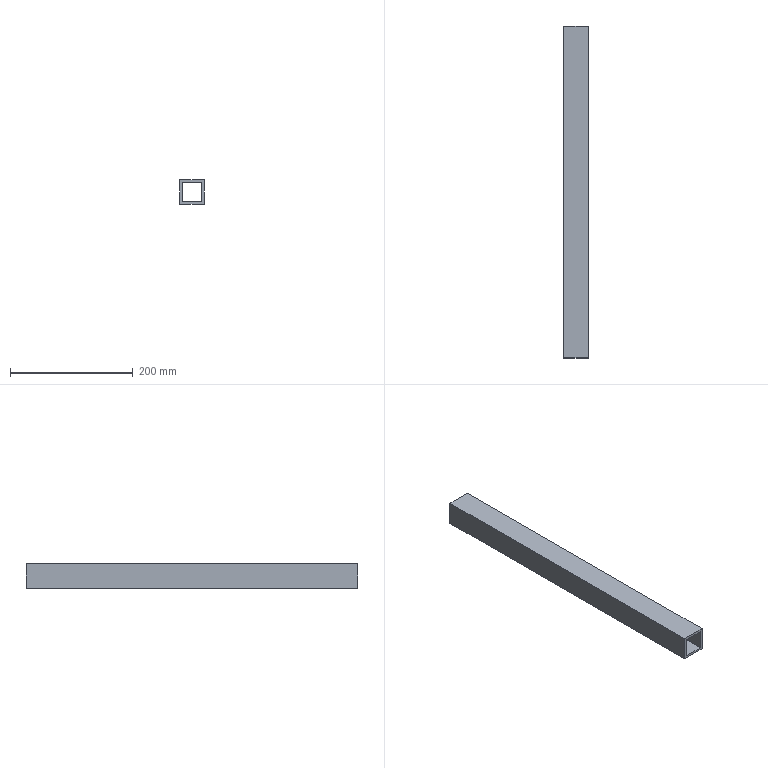Part | NX | features solid 2 | 1 solid | 10 faces | box 40 x 540 x 40 mm | volume 311040 mm3 | plane 10
STEP:
#1=CARTESIAN_POINT('',(-1540.,-370.,-85.));
#2=VERTEX_POINT('',#1);
#3=CARTESIAN_POINT('',(-1540.,170.,-85.));
#4=VERTEX_POINT('',#3);
#5=CARTESIAN_POINT('',(-1540.,1629.393,-85.));
#6=DIRECTION('',(0.,1.,0.));
#7=VECTOR('',#6,1000.);
#8=LINE('',#5,#7);
#9=EDGE_CURVE('',#2,#4,#8,.T.);
#10=ORIENTED_EDGE('',*,*,#9,.T.);
#11=CARTESIAN_POINT('',(-1540.,170.,-45.));
#12=VERTEX_POINT('',#11);
#13=CARTESIAN_POINT('',(-1540.,170.,-70.));
#14=DIRECTION('',(0.,0.,1.));
#15=VECTOR('',#14,1000.);
#16=LINE('',#13,#15);
#17=EDGE_CURVE('',#4,#12,#16,.T.);
#18=ORIENTED_EDGE('',*,*,#17,.T.);
#19=CARTESIAN_POINT('',(-1540.,-370.,-45.));
#20=VERTEX_POINT('',#19);
#21=CARTESIAN_POINT('',(-1540.,1714.393,-45.));
#22=DIRECTION('',(0.,1.,0.));
#23=VECTOR('',#22,1000.);
#24=LINE('',#21,#23);
#25=EDGE_CURVE('',#20,#12,#24,.T.);
#26=ORIENTED_EDGE('',*,*,#25,.F.);
#27=CARTESIAN_POINT('',(-1540.,-370.,-70.));
#28=DIRECTION('',(0.,0.,-1.));
#29=VECTOR('',#28,1000.);
#30=LINE('',#27,#29);
#31=EDGE_CURVE('',#20,#2,#30,.T.);
#32=ORIENTED_EDGE('',*,*,#31,.T.);
#33=EDGE_LOOP('',(#10,#18,#26,#32));
#34=FACE_BOUND('',#33,.T.);
#35=CARTESIAN_POINT('',(-1540.,1629.393,-70.));
#36=DIRECTION('',(-1.,0.,0.));
#37=DIRECTION('',(0.,0.,1.));
#38=AXIS2_PLACEMENT_3D('',#35,#36,#37);
#39=PLANE('',#38);
#40=ADVANCED_FACE('',(#34),#39,.F.);
#41=CARTESIAN_POINT('',(-1580.,-370.,-85.));
#42=VERTEX_POINT('',#41);
#43=CARTESIAN_POINT('',(-1580.,170.,-85.));
#44=VERTEX_POINT('',#43);
#45=CARTESIAN_POINT('',(-1580.,1714.393,-85.));
#46=DIRECTION('',(0.,1.,0.));
#47=VECTOR('',#46,1000.);
#48=LINE('',#45,#47);
#49=EDGE_CURVE('',#42,#44,#48,.T.);
#50=ORIENTED_EDGE('',*,*,#49,.T.);
#51=CARTESIAN_POINT('',(-960.,170.,-85.));
#52=DIRECTION('',(1.,0.,0.));
#53=VECTOR('',#52,1000.);
#54=LINE('',#51,#53);
#55=EDGE_CURVE('',#44,#4,#54,.T.);
#56=ORIENTED_EDGE('',*,*,#55,.T.);
#57=ORIENTED_EDGE('',*,*,#9,.F.);
#58=CARTESIAN_POINT('',(-960.,-370.,-85.));
#59=DIRECTION('',(-1.,0.,0.));
#60=VECTOR('',#59,1000.);
#61=LINE('',#58,#60);
#62=EDGE_CURVE('',#2,#42,#61,.T.);
#63=ORIENTED_EDGE('',*,*,#62,.T.);
#64=EDGE_LOOP('',(#50,#56,#57,#63));
#65=FACE_BOUND('',#64,.T.);
#66=CARTESIAN_POINT('',(-960.,1714.393,-85.));
#67=DIRECTION('',(0.,0.,1.));
#68=DIRECTION('',(1.,0.,0.));
#69=AXIS2_PLACEMENT_3D('',#66,#67,#68);
#70=PLANE('',#69);
#71=ADVANCED_FACE('',(#65),#70,.F.);
#72=ORIENTED_EDGE('',*,*,#25,.T.);
#73=CARTESIAN_POINT('',(-1580.,170.,-45.));
#74=VERTEX_POINT('',#73);
#75=CARTESIAN_POINT('',(-920.,170.,-45.));
#76=DIRECTION('',(-1.,0.,0.));
#77=VECTOR('',#76,1000.);
#78=LINE('',#75,#77);
#79=EDGE_CURVE('',#12,#74,#78,.T.);
#80=ORIENTED_EDGE('',*,*,#79,.T.);
#81=CARTESIAN_POINT('',(-1580.,-370.,-45.));
#82=VERTEX_POINT('',#81);
#83=CARTESIAN_POINT('',(-1580.,1714.393,-45.));
#84=DIRECTION('',(0.,-1.,0.));
#85=VECTOR('',#84,1000.);
#86=LINE('',#83,#85);
#87=EDGE_CURVE('',#74,#82,#86,.T.);
#88=ORIENTED_EDGE('',*,*,#87,.T.);
#89=CARTESIAN_POINT('',(-920.,-370.,-45.));
#90=DIRECTION('',(1.,0.,0.));
#91=VECTOR('',#90,1000.);
#92=LINE('',#89,#91);
#93=EDGE_CURVE('',#82,#20,#92,.T.);
#94=ORIENTED_EDGE('',*,*,#93,.T.);
#95=EDGE_LOOP('',(#72,#80,#88,#94));
#96=FACE_BOUND('',#95,.T.);
#97=CARTESIAN_POINT('',(-920.,1714.393,-45.));
#98=DIRECTION('',(0.,0.,-1.));
#99=DIRECTION('',(-1.,0.,0.));
#100=AXIS2_PLACEMENT_3D('',#97,#98,#99);
#101=PLANE('',#100);
#102=ADVANCED_FACE('',(#96),#101,.F.);
#103=ORIENTED_EDGE('',*,*,#87,.F.);
#104=CARTESIAN_POINT('',(-1580.,170.,-40.));
#105=DIRECTION('',(0.,0.,-1.));
#106=VECTOR('',#105,1000.);
#107=LINE('',#104,#106);
#108=EDGE_CURVE('',#74,#44,#107,.T.);
#109=ORIENTED_EDGE('',*,*,#108,.T.);
#110=ORIENTED_EDGE('',*,*,#49,.F.);
#111=CARTESIAN_POINT('',(-1580.,-370.,-40.));
#112=DIRECTION('',(0.,0.,1.));
#113=VECTOR('',#112,1000.);
#114=LINE('',#111,#113);
#115=EDGE_CURVE('',#42,#82,#114,.T.);
#116=ORIENTED_EDGE('',*,*,#115,.T.);
#117=EDGE_LOOP('',(#103,#109,#110,#116));
#118=FACE_BOUND('',#117,.T.);
#119=CARTESIAN_POINT('',(-1580.,1629.393,-40.));
#120=DIRECTION('',(1.,0.,0.));
#121=DIRECTION('',(0.,0.,-1.));
#122=AXIS2_PLACEMENT_3D('',#119,#120,#121);
#123=PLANE('',#122);
#124=ADVANCED_FACE('',(#118),#123,.F.);
#125=CARTESIAN_POINT('',(-1544.,170.,-81.));
#126=VERTEX_POINT('',#125);
#127=CARTESIAN_POINT('',(-1544.,170.,-49.));
#128=VERTEX_POINT('',#127);
#129=CARTESIAN_POINT('',(-1544.,170.,-70.));
#130=DIRECTION('',(0.,0.,1.));
#131=VECTOR('',#130,1000.);
#132=LINE('',#129,#131);
#133=EDGE_CURVE('',#126,#128,#132,.T.);
#134=ORIENTED_EDGE('',*,*,#133,.F.);
#135=CARTESIAN_POINT('',(-1544.,-370.,-81.));
#136=VERTEX_POINT('',#135);
#137=CARTESIAN_POINT('',(-1544.,1629.393,-81.));
#138=DIRECTION('',(0.,1.,0.));
#139=VECTOR('',#138,1000.);
#140=LINE('',#137,#139);
#141=EDGE_CURVE('',#136,#126,#140,.T.);
#142=ORIENTED_EDGE('',*,*,#141,.F.);
#143=CARTESIAN_POINT('',(-1544.,-370.,-49.));
#144=VERTEX_POINT('',#143);
#145=CARTESIAN_POINT('',(-1544.,-370.,-70.));
#146=DIRECTION('',(0.,0.,-1.));
#147=VECTOR('',#146,1000.);
#148=LINE('',#145,#147);
#149=EDGE_CURVE('',#144,#136,#148,.T.);
#150=ORIENTED_EDGE('',*,*,#149,.F.);
#151=CARTESIAN_POINT('',(-1544.,1714.393,-49.));
#152=DIRECTION('',(0.,1.,0.));
#153=VECTOR('',#152,1000.);
#154=LINE('',#151,#153);
#155=EDGE_CURVE('',#144,#128,#154,.T.);
#156=ORIENTED_EDGE('',*,*,#155,.T.);
#157=EDGE_LOOP('',(#134,#142,#150,#156));
#158=FACE_BOUND('',#157,.T.);
#159=CARTESIAN_POINT('',(-1544.,1629.393,-70.));
#160=DIRECTION('',(-1.,0.,0.));
#161=DIRECTION('',(0.,0.,1.));
#162=AXIS2_PLACEMENT_3D('',#159,#160,#161);
#163=PLANE('',#162);
#164=ADVANCED_FACE('',(#158),#163,.T.);
#165=CARTESIAN_POINT('',(-1576.,170.,-81.));
#166=VERTEX_POINT('',#165);
#167=CARTESIAN_POINT('',(-960.,170.,-81.));
#168=DIRECTION('',(1.,0.,0.));
#169=VECTOR('',#168,1000.);
#170=LINE('',#167,#169);
#171=EDGE_CURVE('',#166,#126,#170,.T.);
#172=ORIENTED_EDGE('',*,*,#171,.F.);
#173=CARTESIAN_POINT('',(-1576.,-370.,-81.));
#174=VERTEX_POINT('',#173);
#175=CARTESIAN_POINT('',(-1576.,1714.393,-81.));
#176=DIRECTION('',(0.,1.,0.));
#177=VECTOR('',#176,1000.);
#178=LINE('',#175,#177);
#179=EDGE_CURVE('',#174,#166,#178,.T.);
#180=ORIENTED_EDGE('',*,*,#179,.F.);
#181=CARTESIAN_POINT('',(-960.,-370.,-81.));
#182=DIRECTION('',(-1.,0.,0.));
#183=VECTOR('',#182,1000.);
#184=LINE('',#181,#183);
#185=EDGE_CURVE('',#136,#174,#184,.T.);
#186=ORIENTED_EDGE('',*,*,#185,.F.);
#187=ORIENTED_EDGE('',*,*,#141,.T.);
#188=EDGE_LOOP('',(#172,#180,#186,#187));
#189=FACE_BOUND('',#188,.T.);
#190=CARTESIAN_POINT('',(-960.,1714.393,-81.));
#191=DIRECTION('',(0.,0.,1.));
#192=DIRECTION('',(1.,0.,0.));
#193=AXIS2_PLACEMENT_3D('',#190,#191,#192);
#194=PLANE('',#193);
#195=ADVANCED_FACE('',(#189),#194,.T.);
#196=CARTESIAN_POINT('',(-1576.,170.,-49.));
#197=VERTEX_POINT('',#196);
#198=CARTESIAN_POINT('',(-920.,170.,-49.));
#199=DIRECTION('',(-1.,0.,0.));
#200=VECTOR('',#199,1000.);
#201=LINE('',#198,#200);
#202=EDGE_CURVE('',#128,#197,#201,.T.);
#203=ORIENTED_EDGE('',*,*,#202,.F.);
#204=ORIENTED_EDGE('',*,*,#155,.F.);
#205=CARTESIAN_POINT('',(-1576.,-370.,-49.));
#206=VERTEX_POINT('',#205);
#207=CARTESIAN_POINT('',(-920.,-370.,-49.));
#208=DIRECTION('',(1.,0.,0.));
#209=VECTOR('',#208,1000.);
#210=LINE('',#207,#209);
#211=EDGE_CURVE('',#206,#144,#210,.T.);
#212=ORIENTED_EDGE('',*,*,#211,.F.);
#213=CARTESIAN_POINT('',(-1576.,1714.393,-49.));
#214=DIRECTION('',(0.,-1.,0.));
#215=VECTOR('',#214,1000.);
#216=LINE('',#213,#215);
#217=EDGE_CURVE('',#197,#206,#216,.T.);
#218=ORIENTED_EDGE('',*,*,#217,.F.);
#219=EDGE_LOOP('',(#203,#204,#212,#218));
#220=FACE_BOUND('',#219,.T.);
#221=CARTESIAN_POINT('',(-920.,1714.393,-49.));
#222=DIRECTION('',(0.,0.,-1.));
#223=DIRECTION('',(-1.,0.,0.));
#224=AXIS2_PLACEMENT_3D('',#221,#222,#223);
#225=PLANE('',#224);
#226=ADVANCED_FACE('',(#220),#225,.T.);
#227=CARTESIAN_POINT('',(-1576.,170.,-40.));
#228=DIRECTION('',(0.,0.,-1.));
#229=VECTOR('',#228,1000.);
#230=LINE('',#227,#229);
#231=EDGE_CURVE('',#197,#166,#230,.T.);
#232=ORIENTED_EDGE('',*,*,#231,.F.);
#233=ORIENTED_EDGE('',*,*,#217,.T.);
#234=CARTESIAN_POINT('',(-1576.,-370.,-40.));
#235=DIRECTION('',(0.,0.,1.));
#236=VECTOR('',#235,1000.);
#237=LINE('',#234,#236);
#238=EDGE_CURVE('',#174,#206,#237,.T.);
#239=ORIENTED_EDGE('',*,*,#238,.F.);
#240=ORIENTED_EDGE('',*,*,#179,.T.);
#241=EDGE_LOOP('',(#232,#233,#239,#240));
#242=FACE_BOUND('',#241,.T.);
#243=CARTESIAN_POINT('',(-1576.,1629.393,-40.));
#244=DIRECTION('',(1.,0.,0.));
#245=DIRECTION('',(0.,0.,-1.));
#246=AXIS2_PLACEMENT_3D('',#243,#244,#245);
#247=PLANE('',#246);
#248=ADVANCED_FACE('',(#242),#247,.T.);
#249=ORIENTED_EDGE('',*,*,#211,.T.);
#250=ORIENTED_EDGE('',*,*,#149,.T.);
#251=ORIENTED_EDGE('',*,*,#185,.T.);
#252=ORIENTED_EDGE('',*,*,#238,.T.);
#253=EDGE_LOOP('',(#249,#250,#251,#252));
#254=FACE_BOUND('',#253,.T.);
#255=ORIENTED_EDGE('',*,*,#31,.F.);
#256=ORIENTED_EDGE('',*,*,#93,.F.);
#257=ORIENTED_EDGE('',*,*,#115,.F.);
#258=ORIENTED_EDGE('',*,*,#62,.F.);
#259=EDGE_LOOP('',(#255,#256,#257,#258));
#260=FACE_BOUND('',#259,.T.);
#261=CARTESIAN_POINT('',(149.393,-370.,-70.));
#262=DIRECTION('',(0.,1.,0.));
#263=DIRECTION('',(0.,0.,1.));
#264=AXIS2_PLACEMENT_3D('',#261,#262,#263);
#265=PLANE('',#264);
#266=ADVANCED_FACE('',(#254,#260),#265,.F.);
#267=ORIENTED_EDGE('',*,*,#133,.T.);
#268=ORIENTED_EDGE('',*,*,#202,.T.);
#269=ORIENTED_EDGE('',*,*,#231,.T.);
#270=ORIENTED_EDGE('',*,*,#171,.T.);
#271=EDGE_LOOP('',(#267,#268,#269,#270));
#272=FACE_BOUND('',#271,.T.);
#273=ORIENTED_EDGE('',*,*,#55,.F.);
#274=ORIENTED_EDGE('',*,*,#108,.F.);
#275=ORIENTED_EDGE('',*,*,#79,.F.);
#276=ORIENTED_EDGE('',*,*,#17,.F.);
#277=EDGE_LOOP('',(#273,#274,#275,#276));
#278=FACE_BOUND('',#277,.T.);
#279=CARTESIAN_POINT('',(149.393,170.,-40.));
#280=DIRECTION('',(0.,-1.,0.));
#281=DIRECTION('',(0.,0.,-1.));
#282=AXIS2_PLACEMENT_3D('',#279,#280,#281);
#283=PLANE('',#282);
#284=ADVANCED_FACE('',(#272,#278),#283,.F.);
#285=CLOSED_SHELL('',(#40,#71,#102,#124,#164,#195,#226,#248,#266,#284));
#286=MANIFOLD_SOLID_BREP('',#285);
#287=(LENGTH_UNIT()NAMED_UNIT(*)SI_UNIT(.MILLI.,.METRE.));
#288=UNCERTAINTY_MEASURE_WITH_UNIT(LENGTH_MEASURE(0.00001),#287,'','');
#289=(NAMED_UNIT(*)PLANE_ANGLE_UNIT()SI_UNIT($,.RADIAN.));
#290=(NAMED_UNIT(*)SI_UNIT($,.STERADIAN.)SOLID_ANGLE_UNIT());
#291=(GEOMETRIC_REPRESENTATION_CONTEXT(3)GLOBAL_UNCERTAINTY_ASSIGNED_CONTEXT((#288))GLOBAL_UNIT_ASSIGNED_CONTEXT((#287,#289,#290))REPRESENTATION_CONTEXT('',''));
#292=ADVANCED_BREP_SHAPE_REPRESENTATION('',(#286),#291);